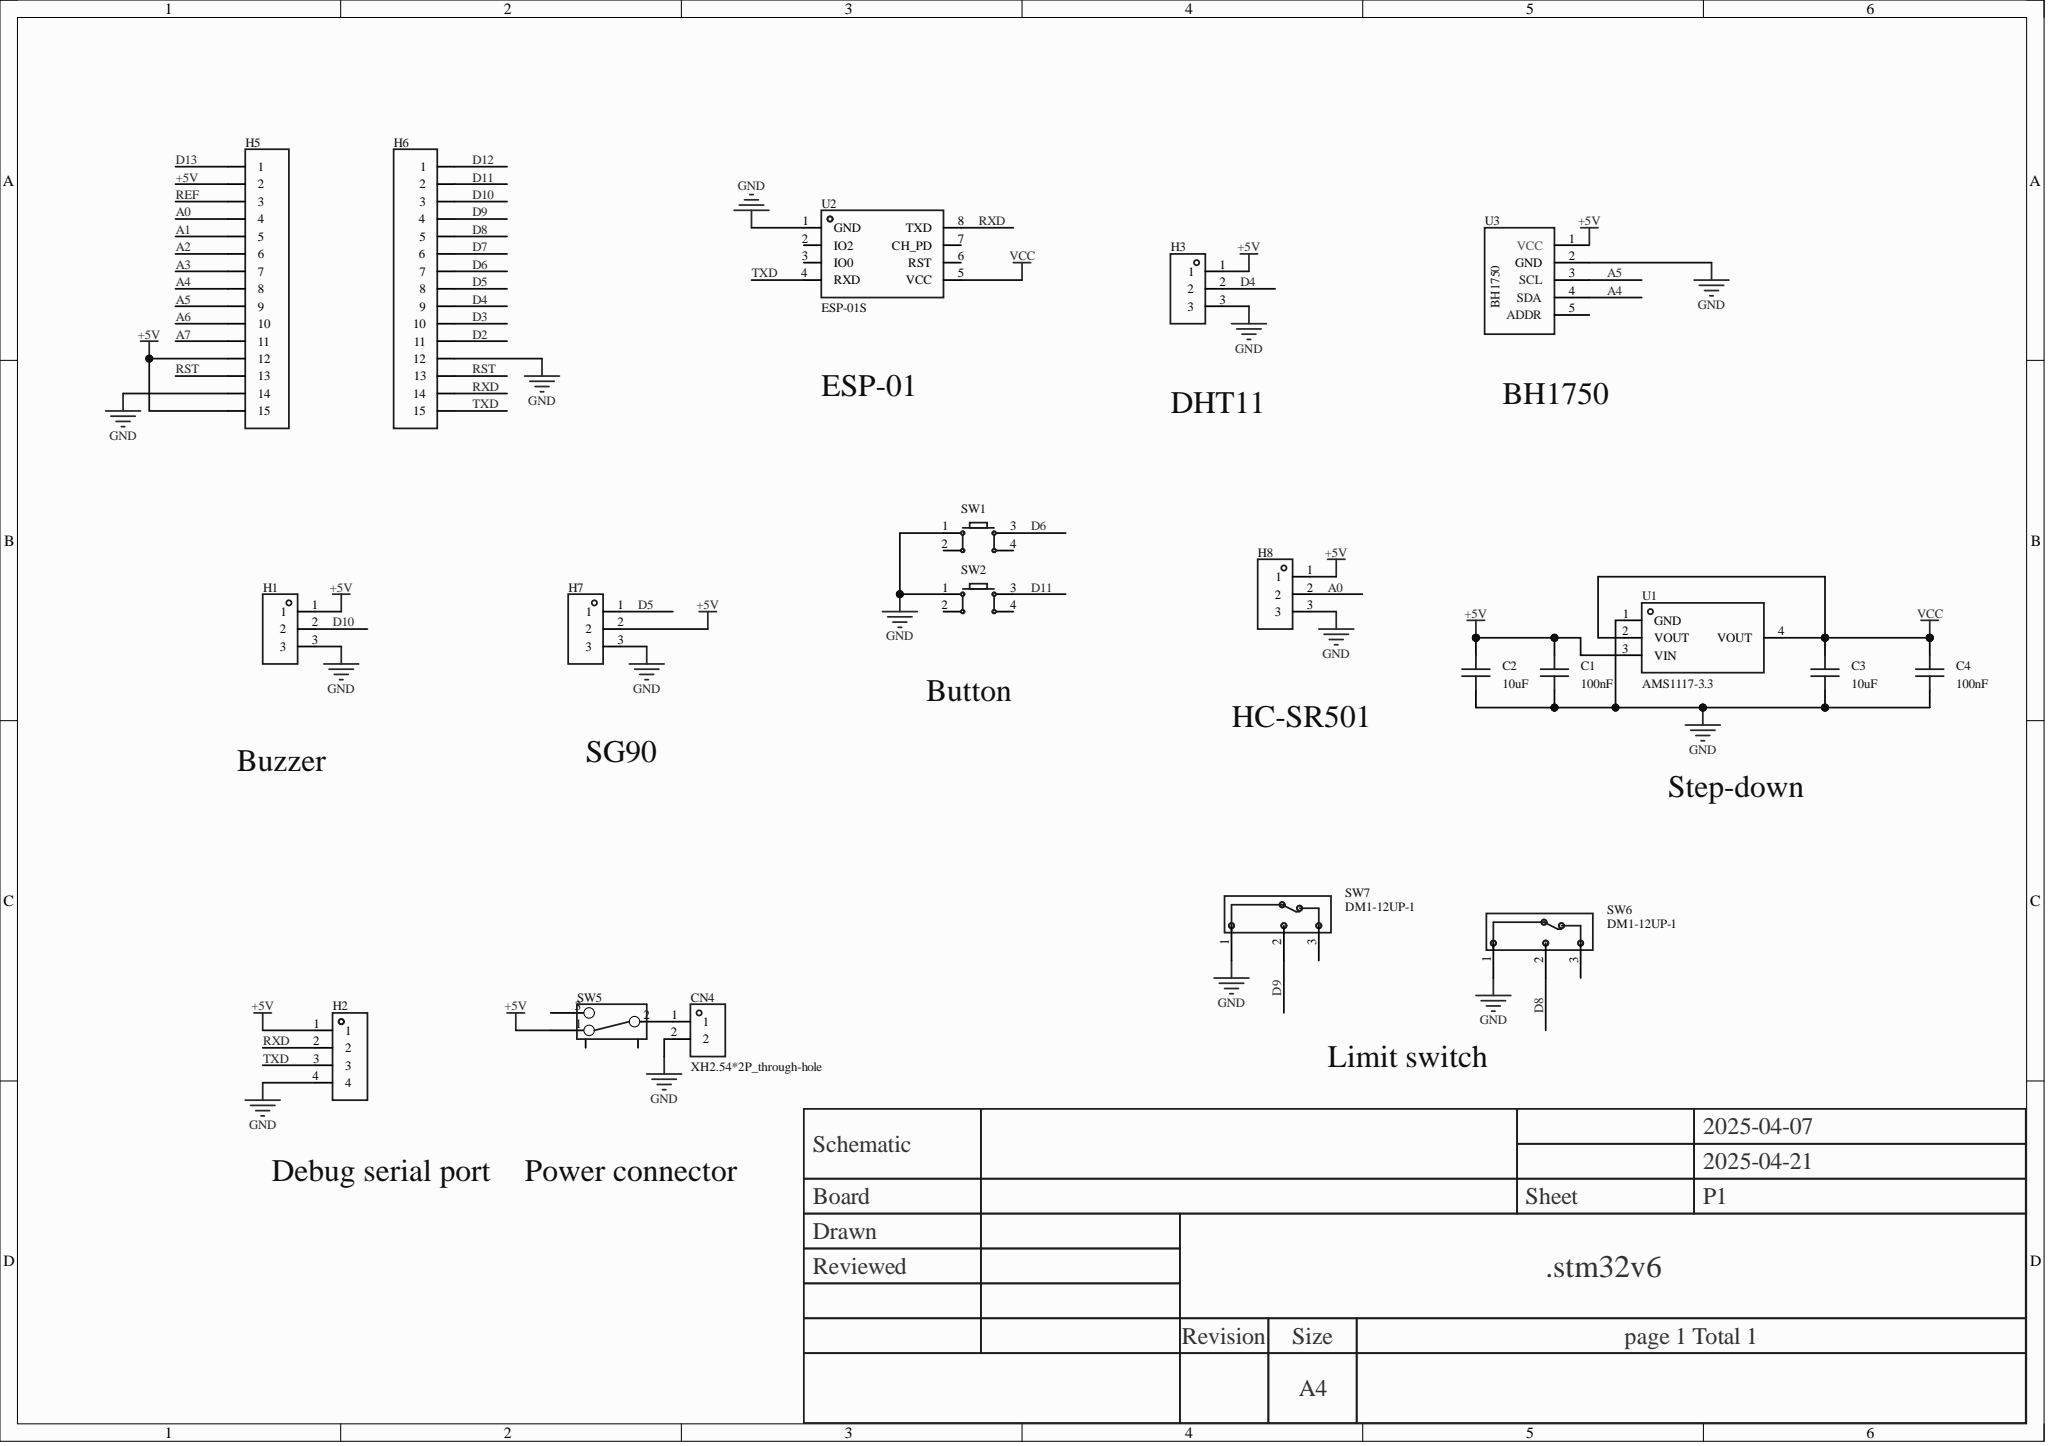Circuit board | Altium Designer | 20 parts | 17 nets
Bill of materials:
Comment,Description,Designator,Footprint,LibRef,Quantity
"100nF","","C1, C4","C0603","CAP_0603","2"
"10uF","","C2, C3","C0603","CAP_0603","2"
"XH2.54*2P_through-hole","","CN4","CONN-TH_2P-P2.50-XH2.54-2P","XH2.54*2P_直插","1"
"","","H1, H3, H7, H8","HDR-TH_3P-P2.54-V-F","HDR-F_2.54_1x3P","4"
"","","H2","HDR-TH_4P-P2.54-V-F","HDR-F_2.54_1x4P","1"
"","","H5, H6","HDR-TH_15P-P2.54-V-F-1","HDR-F_2.54_1x15P","2"
"","","SW1, SW2","SW-TH_4P-L6.0-W6.0-P4.50-LS6.5","Key_TH_6x6x6","2"
"","","SW5","拨动开关","拨动开关_正","1"
"DM1-12UP-1","电路结构:单刀双掷;额定电流(DC):1A;额定电压(DC):30V;额定电流(AC):-;额定电压(AC):-;工作寿命:100万次;","SW6, SW7","SW-TH_DM1-12UP-1","DM1-12UP-1","2"
"AMS1117-3.3","Output type: fixed; operating voltage: -; output voltage: 3.3V; output current: 1A; power supply ripple rejection (PSRR): 72dB@(120Hz); output polarity: positive;","U1","SOT-223-3_L6.5-W3.4-P2.30-LS7.0-BR","AMS1117-3.3_C6186","1"
"ESP-01S","","U2","WIFIM-TH_ESP-01S","ESP-01S_C111009","1"
"","","U3","BH1750光照传感器","BH1750光照传感器","1"
Netlist (Protel format):
[
C1
C0603
100nF



]
[
C2
C0603
10uF



]
[
C3
C0603
10uF



]
[
C4
C0603
100nF



]
[
CN4
CONN-TH_2P-P2.50-XH2.54-2P
XH2.54*2P_through-hole



]
[
H1
HDR-TH_3P-P2.54-V-F




]
[
H2
HDR-TH_4P-P2.54-V-F




]
[
H3
HDR-TH_3P-P2.54-V-F




]
[
H5
HDR-TH_15P-P2.54-V-F-1




]
[
H6
HDR-TH_15P-P2.54-V-F-1




]
[
H7
HDR-TH_3P-P2.54-V-F




]
[
H8
HDR-TH_3P-P2.54-V-F




]
[
SW1
SW-TH_4P-L6.0-W6.0-P4.50-LS6.5




]
[
SW2
SW-TH_4P-L6.0-W6.0-P4.50-LS6.5




]
[
SW5
拨动开关




]
[
SW6
SW-TH_DM1-12UP-1
DM1-12UP-1



]
[
SW7
SW-TH_DM1-12UP-1
DM1-12UP-1



]
[
U1
SOT-223-3_L6.5-W3.4-P2.30-LS7.0-BR
AMS1117-3.3



]
[
U2
WIFIM-TH_ESP-01S
ESP-01S



]
[
U3
BH1750光照传感器




]
(
VCC
C3-2
C4-2
U1-2
U1-4
U2-5
)
(
TXD
H2-3
H6-15
U2-4
)
(
RXD
H2-2
H6-14
U2-8
)
(
RST
H5-13
H6-13
)
(
NetCN4_1
CN4-1
SW5-2
)
(
GND
C1-1
C2-1
C3-1
C4-1
CN4-2
H1-3
H2-4
H3-3
H5-14
H6-12
H7-3
H8-3
SW1-1
SW2-1
SW6-1
SW7-1
U1-1
U2-1
U3-2
)
(
D11
H6-2
SW2-3
)
(
D10
H1-2
H6-3
)
(
D9
H6-4
SW7-2
)
(
D8
H6-5
SW6-2
)
(
D6
H6-7
SW1-3
)
(
D5
H6-8
H7-1
)
(
D4
H3-2
H6-9
)
(
A5
H5-9
U3-3
)
(
A4
H5-8
U3-4
)
(
A0
H5-4
H8-2
)
(
+5V
C1-2
C2-2
H1-1
H2-1
H3-1
H5-2
H5-12
H5-15
H7-2
H8-1
SW5-1
U1-3
U3-1
)